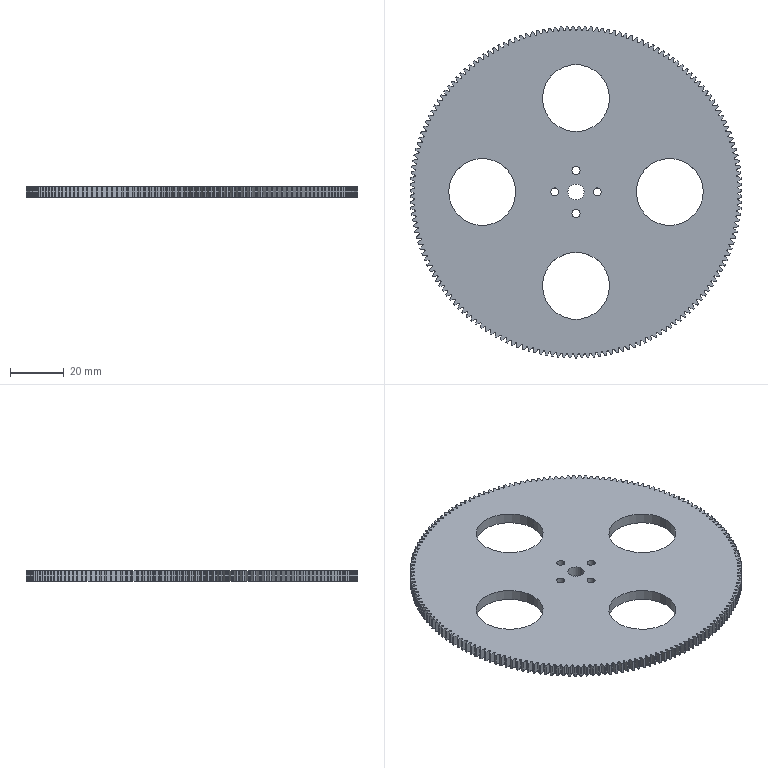Part | SolidWorks | features ICE 2, CirPattern 1, Extrusion 1, RefAxis 1 | 1 solid | 720 faces | box 123.899 x 123.895 x 4 mm | volume 39033 mm3 | cylinder 368 | spline 350 | plane 2 | commonest cylinder face diameters 120.75 x175 123.9 x175 3 x8 25 x8 6 x2